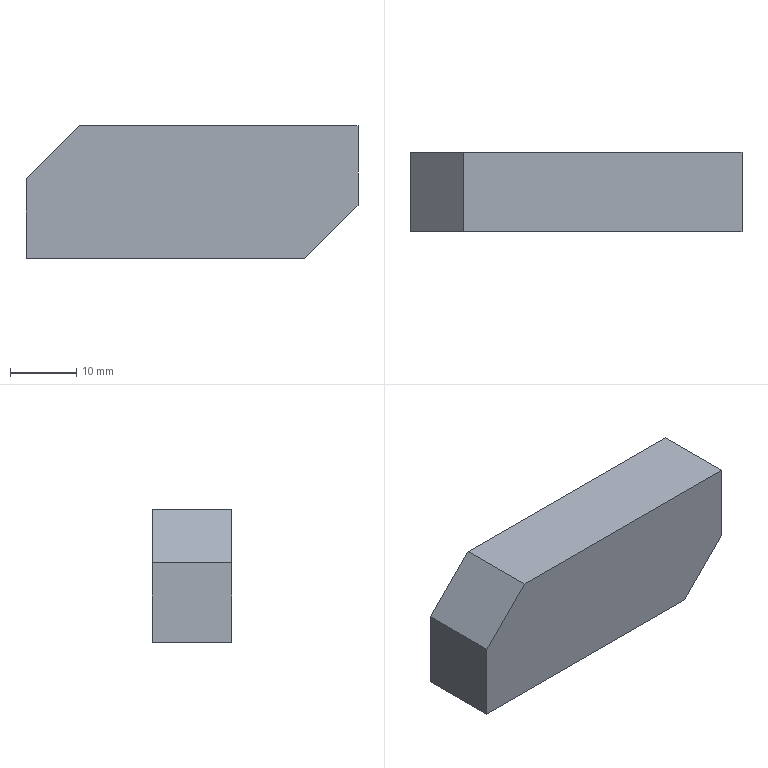Part | NX | features DATUM_CSYS 2, EXTRUDE 1, SKETCH 1 | 1 solid | 8 faces | box 50 x 12 x 20 mm | volume 11232 mm3 | plane 8
STEP:
#1=CARTESIAN_POINT('',(-25.,0.,2.));
#2=VERTEX_POINT('',#1);
#3=CARTESIAN_POINT('',(-25.,0.,-10.));
#4=VERTEX_POINT('',#3);
#5=CARTESIAN_POINT('',(-25.,0.,2.));
#6=DIRECTION('',(0.,0.,-1.));
#7=VECTOR('',#6,1000.);
#8=LINE('',#5,#7);
#9=EDGE_CURVE('',#2,#4,#8,.T.);
#10=ORIENTED_EDGE('',*,*,#9,.T.);
#11=CARTESIAN_POINT('',(-25.,-12.,-10.));
#12=VERTEX_POINT('',#11);
#13=CARTESIAN_POINT('',(-25.,-12.,-10.));
#14=DIRECTION('',(0.,1.,0.));
#15=VECTOR('',#14,1000.);
#16=LINE('',#13,#15);
#17=EDGE_CURVE('',#12,#4,#16,.T.);
#18=ORIENTED_EDGE('',*,*,#17,.F.);
#19=CARTESIAN_POINT('',(-25.,-12.,2.));
#20=VERTEX_POINT('',#19);
#21=CARTESIAN_POINT('',(-25.,-12.,2.));
#22=DIRECTION('',(0.,0.,-1.));
#23=VECTOR('',#22,1000.);
#24=LINE('',#21,#23);
#25=EDGE_CURVE('',#20,#12,#24,.T.);
#26=ORIENTED_EDGE('',*,*,#25,.F.);
#27=CARTESIAN_POINT('',(-25.,-12.,2.));
#28=DIRECTION('',(0.,1.,0.));
#29=VECTOR('',#28,1000.);
#30=LINE('',#27,#29);
#31=EDGE_CURVE('',#20,#2,#30,.T.);
#32=ORIENTED_EDGE('',*,*,#31,.T.);
#33=EDGE_LOOP('',(#10,#18,#26,#32));
#34=FACE_BOUND('',#33,.T.);
#35=CARTESIAN_POINT('',(-25.,-12.,2.));
#36=DIRECTION('',(1.,0.,0.));
#37=DIRECTION('',(0.,0.,-1.));
#38=AXIS2_PLACEMENT_3D('',#35,#36,#37);
#39=PLANE('',#38);
#40=ADVANCED_FACE('',(#34),#39,.F.);
#41=CARTESIAN_POINT('',(17.,0.,-10.));
#42=VERTEX_POINT('',#41);
#43=CARTESIAN_POINT('',(-25.,0.,-10.));
#44=DIRECTION('',(1.,0.,0.));
#45=VECTOR('',#44,1000.);
#46=LINE('',#43,#45);
#47=EDGE_CURVE('',#4,#42,#46,.T.);
#48=ORIENTED_EDGE('',*,*,#47,.T.);
#49=CARTESIAN_POINT('',(17.,-12.,-10.));
#50=VERTEX_POINT('',#49);
#51=CARTESIAN_POINT('',(17.,-12.,-10.));
#52=DIRECTION('',(0.,1.,0.));
#53=VECTOR('',#52,1000.);
#54=LINE('',#51,#53);
#55=EDGE_CURVE('',#50,#42,#54,.T.);
#56=ORIENTED_EDGE('',*,*,#55,.F.);
#57=CARTESIAN_POINT('',(-25.,-12.,-10.));
#58=DIRECTION('',(1.,0.,0.));
#59=VECTOR('',#58,1000.);
#60=LINE('',#57,#59);
#61=EDGE_CURVE('',#12,#50,#60,.T.);
#62=ORIENTED_EDGE('',*,*,#61,.F.);
#63=ORIENTED_EDGE('',*,*,#17,.T.);
#64=EDGE_LOOP('',(#48,#56,#62,#63));
#65=FACE_BOUND('',#64,.T.);
#66=CARTESIAN_POINT('',(-25.,-12.,-10.));
#67=DIRECTION('',(0.,0.,1.));
#68=DIRECTION('',(1.,0.,0.));
#69=AXIS2_PLACEMENT_3D('',#66,#67,#68);
#70=PLANE('',#69);
#71=ADVANCED_FACE('',(#65),#70,.F.);
#72=CARTESIAN_POINT('',(25.,0.,-2.));
#73=VERTEX_POINT('',#72);
#74=CARTESIAN_POINT('',(17.,0.,-10.));
#75=DIRECTION('',(0.7071,0.,0.7071));
#76=VECTOR('',#75,1000.);
#77=LINE('',#74,#76);
#78=EDGE_CURVE('',#42,#73,#77,.T.);
#79=ORIENTED_EDGE('',*,*,#78,.T.);
#80=CARTESIAN_POINT('',(25.,-12.,-2.));
#81=VERTEX_POINT('',#80);
#82=CARTESIAN_POINT('',(25.,-12.,-2.));
#83=DIRECTION('',(0.,1.,0.));
#84=VECTOR('',#83,1000.);
#85=LINE('',#82,#84);
#86=EDGE_CURVE('',#81,#73,#85,.T.);
#87=ORIENTED_EDGE('',*,*,#86,.F.);
#88=CARTESIAN_POINT('',(17.,-12.,-10.));
#89=DIRECTION('',(0.7071,0.,0.7071));
#90=VECTOR('',#89,1000.);
#91=LINE('',#88,#90);
#92=EDGE_CURVE('',#50,#81,#91,.T.);
#93=ORIENTED_EDGE('',*,*,#92,.F.);
#94=ORIENTED_EDGE('',*,*,#55,.T.);
#95=EDGE_LOOP('',(#79,#87,#93,#94));
#96=FACE_BOUND('',#95,.T.);
#97=CARTESIAN_POINT('',(17.,-12.,-10.));
#98=DIRECTION('',(-0.7071,0.,0.7071));
#99=DIRECTION('',(0.7071,0.,0.7071));
#100=AXIS2_PLACEMENT_3D('',#97,#98,#99);
#101=PLANE('',#100);
#102=ADVANCED_FACE('',(#96),#101,.F.);
#103=CARTESIAN_POINT('',(25.,0.,10.));
#104=VERTEX_POINT('',#103);
#105=CARTESIAN_POINT('',(25.,0.,-2.));
#106=DIRECTION('',(0.,0.,1.));
#107=VECTOR('',#106,1000.);
#108=LINE('',#105,#107);
#109=EDGE_CURVE('',#73,#104,#108,.T.);
#110=ORIENTED_EDGE('',*,*,#109,.T.);
#111=CARTESIAN_POINT('',(25.,-12.,10.));
#112=VERTEX_POINT('',#111);
#113=CARTESIAN_POINT('',(25.,-12.,10.));
#114=DIRECTION('',(0.,1.,0.));
#115=VECTOR('',#114,1000.);
#116=LINE('',#113,#115);
#117=EDGE_CURVE('',#112,#104,#116,.T.);
#118=ORIENTED_EDGE('',*,*,#117,.F.);
#119=CARTESIAN_POINT('',(25.,-12.,-2.));
#120=DIRECTION('',(0.,0.,1.));
#121=VECTOR('',#120,1000.);
#122=LINE('',#119,#121);
#123=EDGE_CURVE('',#81,#112,#122,.T.);
#124=ORIENTED_EDGE('',*,*,#123,.F.);
#125=ORIENTED_EDGE('',*,*,#86,.T.);
#126=EDGE_LOOP('',(#110,#118,#124,#125));
#127=FACE_BOUND('',#126,.T.);
#128=CARTESIAN_POINT('',(25.,-12.,-2.));
#129=DIRECTION('',(-1.,0.,0.));
#130=DIRECTION('',(0.,0.,1.));
#131=AXIS2_PLACEMENT_3D('',#128,#129,#130);
#132=PLANE('',#131);
#133=ADVANCED_FACE('',(#127),#132,.F.);
#134=CARTESIAN_POINT('',(-17.,0.,10.));
#135=VERTEX_POINT('',#134);
#136=CARTESIAN_POINT('',(25.,0.,10.));
#137=DIRECTION('',(-1.,0.,0.));
#138=VECTOR('',#137,1000.);
#139=LINE('',#136,#138);
#140=EDGE_CURVE('',#104,#135,#139,.T.);
#141=ORIENTED_EDGE('',*,*,#140,.T.);
#142=CARTESIAN_POINT('',(-17.,-12.,10.));
#143=VERTEX_POINT('',#142);
#144=CARTESIAN_POINT('',(-17.,-12.,10.));
#145=DIRECTION('',(0.,1.,0.));
#146=VECTOR('',#145,1000.);
#147=LINE('',#144,#146);
#148=EDGE_CURVE('',#143,#135,#147,.T.);
#149=ORIENTED_EDGE('',*,*,#148,.F.);
#150=CARTESIAN_POINT('',(25.,-12.,10.));
#151=DIRECTION('',(-1.,0.,0.));
#152=VECTOR('',#151,1000.);
#153=LINE('',#150,#152);
#154=EDGE_CURVE('',#112,#143,#153,.T.);
#155=ORIENTED_EDGE('',*,*,#154,.F.);
#156=ORIENTED_EDGE('',*,*,#117,.T.);
#157=EDGE_LOOP('',(#141,#149,#155,#156));
#158=FACE_BOUND('',#157,.T.);
#159=CARTESIAN_POINT('',(25.,-12.,10.));
#160=DIRECTION('',(0.,0.,-1.));
#161=DIRECTION('',(-1.,0.,0.));
#162=AXIS2_PLACEMENT_3D('',#159,#160,#161);
#163=PLANE('',#162);
#164=ADVANCED_FACE('',(#158),#163,.F.);
#165=CARTESIAN_POINT('',(-17.,0.,10.));
#166=DIRECTION('',(-0.7071,0.,-0.7071));
#167=VECTOR('',#166,1000.);
#168=LINE('',#165,#167);
#169=EDGE_CURVE('',#135,#2,#168,.T.);
#170=ORIENTED_EDGE('',*,*,#169,.T.);
#171=ORIENTED_EDGE('',*,*,#31,.F.);
#172=CARTESIAN_POINT('',(-17.,-12.,10.));
#173=DIRECTION('',(-0.7071,0.,-0.7071));
#174=VECTOR('',#173,1000.);
#175=LINE('',#172,#174);
#176=EDGE_CURVE('',#143,#20,#175,.T.);
#177=ORIENTED_EDGE('',*,*,#176,.F.);
#178=ORIENTED_EDGE('',*,*,#148,.T.);
#179=EDGE_LOOP('',(#170,#171,#177,#178));
#180=FACE_BOUND('',#179,.T.);
#181=CARTESIAN_POINT('',(-17.,-12.,10.));
#182=DIRECTION('',(0.7071,0.,-0.7071));
#183=DIRECTION('',(-0.7071,0.,-0.7071));
#184=AXIS2_PLACEMENT_3D('',#181,#182,#183);
#185=PLANE('',#184);
#186=ADVANCED_FACE('',(#180),#185,.F.);
#187=ORIENTED_EDGE('',*,*,#25,.T.);
#188=ORIENTED_EDGE('',*,*,#61,.T.);
#189=ORIENTED_EDGE('',*,*,#92,.T.);
#190=ORIENTED_EDGE('',*,*,#123,.T.);
#191=ORIENTED_EDGE('',*,*,#154,.T.);
#192=ORIENTED_EDGE('',*,*,#176,.T.);
#193=EDGE_LOOP('',(#187,#188,#189,#190,#191,#192));
#194=FACE_BOUND('',#193,.T.);
#195=CARTESIAN_POINT('',(0.,-12.,0.));
#196=DIRECTION('',(0.,-1.,0.));
#197=DIRECTION('',(0.,0.,-1.));
#198=AXIS2_PLACEMENT_3D('',#195,#196,#197);
#199=PLANE('',#198);
#200=ADVANCED_FACE('',(#194),#199,.T.);
#201=ORIENTED_EDGE('',*,*,#9,.F.);
#202=ORIENTED_EDGE('',*,*,#169,.F.);
#203=ORIENTED_EDGE('',*,*,#140,.F.);
#204=ORIENTED_EDGE('',*,*,#109,.F.);
#205=ORIENTED_EDGE('',*,*,#78,.F.);
#206=ORIENTED_EDGE('',*,*,#47,.F.);
#207=EDGE_LOOP('',(#201,#202,#203,#204,#205,#206));
#208=FACE_BOUND('',#207,.T.);
#209=CARTESIAN_POINT('',(0.,0.,0.));
#210=DIRECTION('',(0.,-1.,0.));
#211=DIRECTION('',(0.,0.,-1.));
#212=AXIS2_PLACEMENT_3D('',#209,#210,#211);
#213=PLANE('',#212);
#214=ADVANCED_FACE('',(#208),#213,.F.);
#215=CLOSED_SHELL('',(#40,#71,#102,#133,#164,#186,#200,#214));
#216=MANIFOLD_SOLID_BREP('',#215);
#217=(LENGTH_UNIT()NAMED_UNIT(*)SI_UNIT(.MILLI.,.METRE.));
#218=UNCERTAINTY_MEASURE_WITH_UNIT(LENGTH_MEASURE(0.00001),#217,'','');
#219=(NAMED_UNIT(*)PLANE_ANGLE_UNIT()SI_UNIT($,.RADIAN.));
#220=(NAMED_UNIT(*)SI_UNIT($,.STERADIAN.)SOLID_ANGLE_UNIT());
#221=(GEOMETRIC_REPRESENTATION_CONTEXT(3)GLOBAL_UNCERTAINTY_ASSIGNED_CONTEXT((#218))GLOBAL_UNIT_ASSIGNED_CONTEXT((#217,#219,#220))REPRESENTATION_CONTEXT('',''));
#222=ADVANCED_BREP_SHAPE_REPRESENTATION('',(#216),#221);